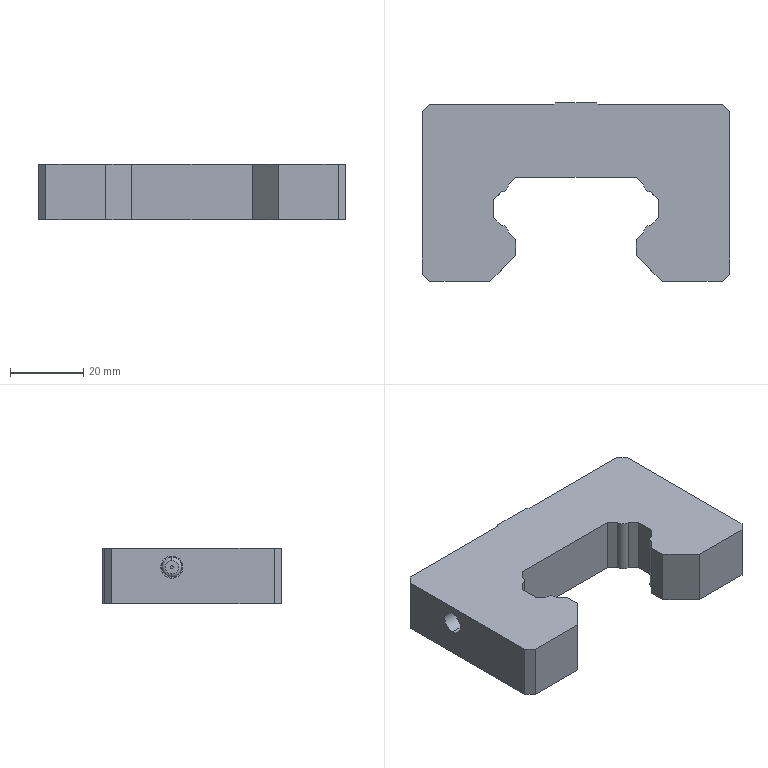Part | SolidWorks | features SplitBody 1 | 1 solid | 57 faces | box 84.105 x 48.965 x 15.15 mm | volume 44523 mm3 | plane 37 | cylinder 16 | torus 4 | commonest cylinder face diameters 3.924 x6 6.06 x6 0.818 x4